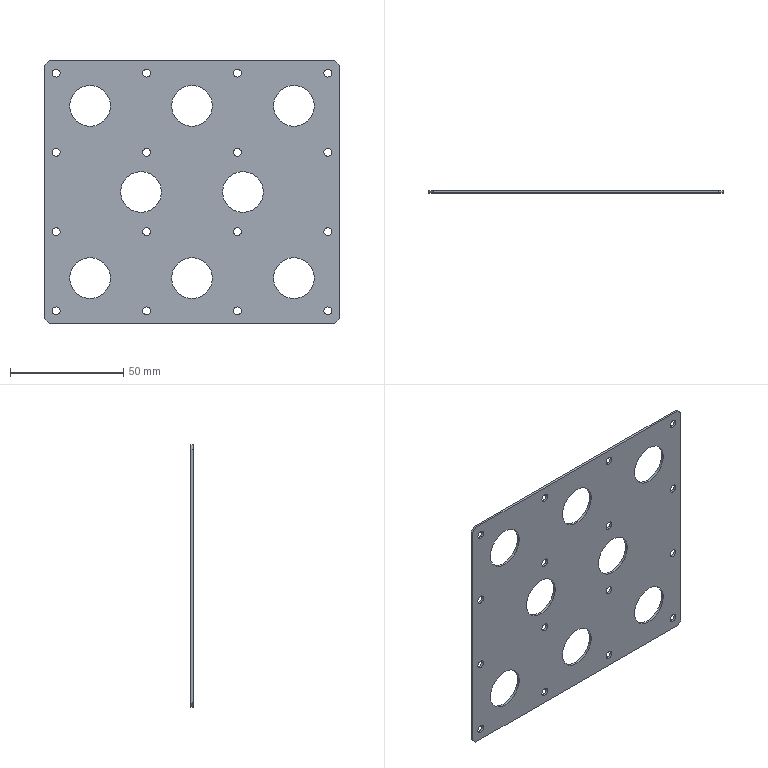Part | SolidWorks | features LPattern 2, Chamfer 1, Extrusion 1, HoleWzd 1, ICE 1 | 1 solid | 58 faces | box 130 x 1 x 116 mm | volume 12882 mm3 | cylinder 48 | plane 10 | commonest cylinder face diameters 3.5 x32 18 x16